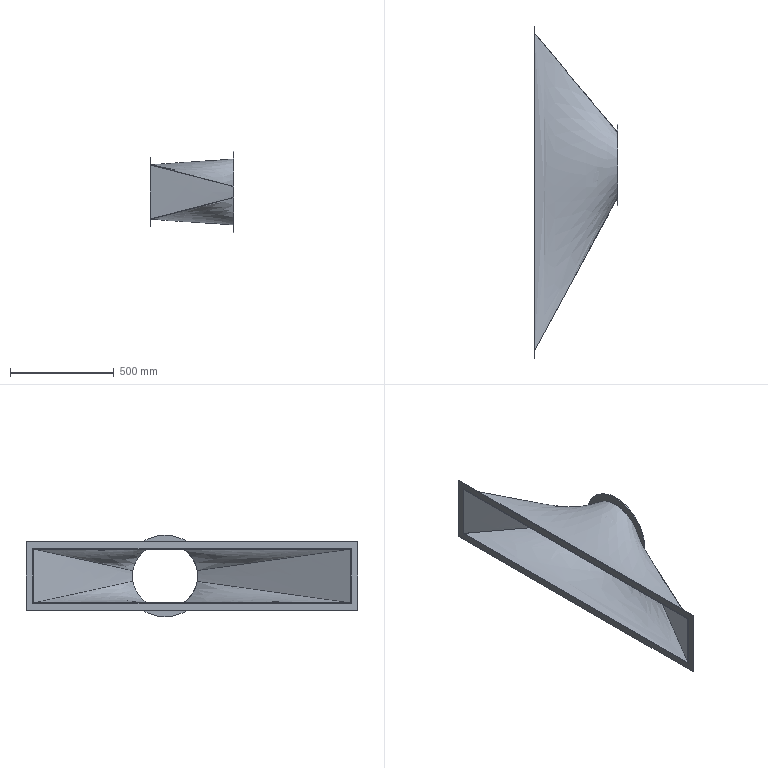Part | STEP file | Produce dryer line heating fan-OVEN-401 | 2 solids | 25 faces | box 403.502 x 1600 x 395 mm | volume 2039591 mm3 | plane 13 | spline 8 | cylinder 4 | commonest cylinder face diameters 315 x2 395 x2